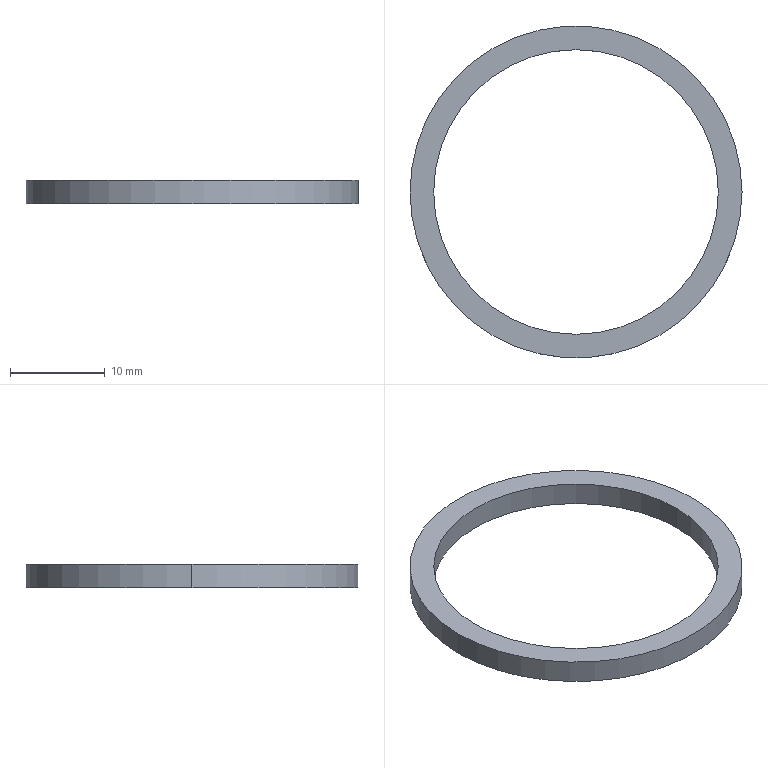Part | SolidWorks | features Extrusion 1 | 1 solid | 6 faces | box 35 x 35 x 2.5 mm | volume 638.136 mm3 | cylinder 4 | plane 2 | commonest cylinder face diameters 30 x2 35 x2
STEP:
#1=CARTESIAN_POINT('',(-15.,0.,2.5));
#2=VERTEX_POINT('',#1);
#3=CARTESIAN_POINT('',(15.,0.,2.5));
#4=VERTEX_POINT('',#3);
#5=CARTESIAN_POINT('',(0.,0.,2.5));
#6=DIRECTION('',(0.,0.,1.));
#7=DIRECTION('',(1.,0.,0.));
#8=AXIS2_PLACEMENT_3D('',#5,#6,#7);
#9=CIRCLE('',#8,15.);
#10=EDGE_CURVE('',#2,#4,#9,.T.);
#11=ORIENTED_EDGE('',*,*,#10,.T.);
#12=CARTESIAN_POINT('',(15.,0.,0.));
#13=VERTEX_POINT('',#12);
#14=CARTESIAN_POINT('',(15.,0.,2.5));
#15=DIRECTION('',(0.,0.,-1.));
#16=VECTOR('',#15,1000.);
#17=LINE('',#14,#16);
#18=EDGE_CURVE('',#4,#13,#17,.T.);
#19=ORIENTED_EDGE('',*,*,#18,.T.);
#20=CARTESIAN_POINT('',(-15.,0.,0.));
#21=VERTEX_POINT('',#20);
#22=CARTESIAN_POINT('',(0.,0.,0.));
#23=DIRECTION('',(0.,0.,1.));
#24=DIRECTION('',(1.,0.,0.));
#25=AXIS2_PLACEMENT_3D('',#22,#23,#24);
#26=CIRCLE('',#25,15.);
#27=EDGE_CURVE('',#21,#13,#26,.T.);
#28=ORIENTED_EDGE('',*,*,#27,.F.);
#29=CARTESIAN_POINT('',(-15.,0.,2.5));
#30=DIRECTION('',(0.,0.,-1.));
#31=VECTOR('',#30,1000.);
#32=LINE('',#29,#31);
#33=EDGE_CURVE('',#2,#21,#32,.T.);
#34=ORIENTED_EDGE('',*,*,#33,.F.);
#35=EDGE_LOOP('',(#11,#19,#28,#34));
#36=FACE_OUTER_BOUND('',#35,.T.);
#37=CARTESIAN_POINT('',(0.,0.,2.5));
#38=DIRECTION('',(0.,0.,-1.));
#39=DIRECTION('',(-1.,0.,0.));
#40=AXIS2_PLACEMENT_3D('',#37,#38,#39);
#41=CYLINDRICAL_SURFACE('',#40,15.);
#42=ADVANCED_FACE('',(#36),#41,.F.);
#43=CARTESIAN_POINT('',(17.5,0.,2.5));
#44=VERTEX_POINT('',#43);
#45=CARTESIAN_POINT('',(-17.5,0.,2.5));
#46=VERTEX_POINT('',#45);
#47=CARTESIAN_POINT('',(0.,0.,2.5));
#48=DIRECTION('',(0.,0.,1.));
#49=DIRECTION('',(1.,0.,0.));
#50=AXIS2_PLACEMENT_3D('',#47,#48,#49);
#51=CIRCLE('',#50,17.5);
#52=EDGE_CURVE('',#44,#46,#51,.T.);
#53=ORIENTED_EDGE('',*,*,#52,.F.);
#54=CARTESIAN_POINT('',(17.5,0.,0.));
#55=VERTEX_POINT('',#54);
#56=CARTESIAN_POINT('',(17.5,0.,2.5));
#57=DIRECTION('',(0.,0.,-1.));
#58=VECTOR('',#57,1000.);
#59=LINE('',#56,#58);
#60=EDGE_CURVE('',#44,#55,#59,.T.);
#61=ORIENTED_EDGE('',*,*,#60,.T.);
#62=CARTESIAN_POINT('',(-17.5,0.,0.));
#63=VERTEX_POINT('',#62);
#64=CARTESIAN_POINT('',(0.,0.,0.));
#65=DIRECTION('',(0.,0.,1.));
#66=DIRECTION('',(1.,0.,0.));
#67=AXIS2_PLACEMENT_3D('',#64,#65,#66);
#68=CIRCLE('',#67,17.5);
#69=EDGE_CURVE('',#55,#63,#68,.T.);
#70=ORIENTED_EDGE('',*,*,#69,.T.);
#71=CARTESIAN_POINT('',(-17.5,0.,2.5));
#72=DIRECTION('',(0.,0.,-1.));
#73=VECTOR('',#72,1000.);
#74=LINE('',#71,#73);
#75=EDGE_CURVE('',#46,#63,#74,.T.);
#76=ORIENTED_EDGE('',*,*,#75,.F.);
#77=EDGE_LOOP('',(#53,#61,#70,#76));
#78=FACE_OUTER_BOUND('',#77,.T.);
#79=CARTESIAN_POINT('',(0.,0.,2.5));
#80=DIRECTION('',(0.,0.,-1.));
#81=DIRECTION('',(-1.,0.,0.));
#82=AXIS2_PLACEMENT_3D('',#79,#80,#81);
#83=CYLINDRICAL_SURFACE('',#82,17.5);
#84=ADVANCED_FACE('',(#78),#83,.T.);
#85=CARTESIAN_POINT('',(0.,0.,2.5));
#86=DIRECTION('',(0.,0.,1.));
#87=DIRECTION('',(1.,0.,0.));
#88=AXIS2_PLACEMENT_3D('',#85,#86,#87);
#89=CIRCLE('',#88,17.5);
#90=EDGE_CURVE('',#46,#44,#89,.T.);
#91=ORIENTED_EDGE('',*,*,#90,.T.);
#92=ORIENTED_EDGE('',*,*,#52,.T.);
#93=EDGE_LOOP('',(#91,#92));
#94=FACE_OUTER_BOUND('',#93,.T.);
#95=ORIENTED_EDGE('',*,*,#10,.F.);
#96=CARTESIAN_POINT('',(0.,0.,2.5));
#97=DIRECTION('',(0.,0.,1.));
#98=DIRECTION('',(1.,0.,0.));
#99=AXIS2_PLACEMENT_3D('',#96,#97,#98);
#100=CIRCLE('',#99,15.);
#101=EDGE_CURVE('',#4,#2,#100,.T.);
#102=ORIENTED_EDGE('',*,*,#101,.F.);
#103=EDGE_LOOP('',(#95,#102));
#104=FACE_BOUND('',#103,.T.);
#105=CARTESIAN_POINT('',(0.,0.,2.5));
#106=DIRECTION('',(0.,0.,1.));
#107=DIRECTION('',(1.,0.,0.));
#108=AXIS2_PLACEMENT_3D('',#105,#106,#107);
#109=PLANE('',#108);
#110=ADVANCED_FACE('',(#94,#104),#109,.T.);
#111=CARTESIAN_POINT('',(0.,0.,0.));
#112=DIRECTION('',(0.,0.,1.));
#113=DIRECTION('',(1.,0.,0.));
#114=AXIS2_PLACEMENT_3D('',#111,#112,#113);
#115=CIRCLE('',#114,17.5);
#116=EDGE_CURVE('',#63,#55,#115,.T.);
#117=ORIENTED_EDGE('',*,*,#116,.F.);
#118=ORIENTED_EDGE('',*,*,#69,.F.);
#119=EDGE_LOOP('',(#117,#118));
#120=FACE_OUTER_BOUND('',#119,.T.);
#121=ORIENTED_EDGE('',*,*,#27,.T.);
#122=CARTESIAN_POINT('',(0.,0.,0.));
#123=DIRECTION('',(0.,0.,1.));
#124=DIRECTION('',(1.,0.,0.));
#125=AXIS2_PLACEMENT_3D('',#122,#123,#124);
#126=CIRCLE('',#125,15.);
#127=EDGE_CURVE('',#13,#21,#126,.T.);
#128=ORIENTED_EDGE('',*,*,#127,.T.);
#129=EDGE_LOOP('',(#121,#128));
#130=FACE_BOUND('',#129,.T.);
#131=CARTESIAN_POINT('',(0.,0.,0.));
#132=DIRECTION('',(0.,0.,1.));
#133=DIRECTION('',(1.,0.,0.));
#134=AXIS2_PLACEMENT_3D('',#131,#132,#133);
#135=PLANE('',#134);
#136=ADVANCED_FACE('',(#120,#130),#135,.F.);
#137=ORIENTED_EDGE('',*,*,#60,.F.);
#138=ORIENTED_EDGE('',*,*,#90,.F.);
#139=ORIENTED_EDGE('',*,*,#75,.T.);
#140=ORIENTED_EDGE('',*,*,#116,.T.);
#141=EDGE_LOOP('',(#137,#138,#139,#140));
#142=FACE_OUTER_BOUND('',#141,.T.);
#143=CARTESIAN_POINT('',(0.,0.,2.5));
#144=DIRECTION('',(0.,0.,-1.));
#145=DIRECTION('',(-1.,0.,0.));
#146=AXIS2_PLACEMENT_3D('',#143,#144,#145);
#147=CYLINDRICAL_SURFACE('',#146,17.5);
#148=ADVANCED_FACE('',(#142),#147,.T.);
#149=ORIENTED_EDGE('',*,*,#18,.F.);
#150=ORIENTED_EDGE('',*,*,#101,.T.);
#151=ORIENTED_EDGE('',*,*,#33,.T.);
#152=ORIENTED_EDGE('',*,*,#127,.F.);
#153=EDGE_LOOP('',(#149,#150,#151,#152));
#154=FACE_OUTER_BOUND('',#153,.T.);
#155=CARTESIAN_POINT('',(0.,0.,2.5));
#156=DIRECTION('',(0.,0.,-1.));
#157=DIRECTION('',(-1.,0.,0.));
#158=AXIS2_PLACEMENT_3D('',#155,#156,#157);
#159=CYLINDRICAL_SURFACE('',#158,15.);
#160=ADVANCED_FACE('',(#154),#159,.F.);
#161=CLOSED_SHELL('',(#42,#84,#110,#136,#148,#160));
#162=MANIFOLD_SOLID_BREP('',#161);
#163=CARTESIAN_POINT('',(0.,0.,0.));
#164=DIRECTION('',(0.,0.,1.));
#165=DIRECTION('',(1.,0.,0.));
#166=AXIS2_PLACEMENT_3D('',#163,#164,#165);
#167=(LENGTH_UNIT()NAMED_UNIT(*)SI_UNIT(.MILLI.,.METRE.));
#168=UNCERTAINTY_MEASURE_WITH_UNIT(LENGTH_MEASURE(0.00001),#167,'','');
#169=(NAMED_UNIT(*)PLANE_ANGLE_UNIT()SI_UNIT($,.RADIAN.));
#170=(NAMED_UNIT(*)SI_UNIT($,.STERADIAN.)SOLID_ANGLE_UNIT());
#171=(GEOMETRIC_REPRESENTATION_CONTEXT(3)GLOBAL_UNCERTAINTY_ASSIGNED_CONTEXT((#168))GLOBAL_UNIT_ASSIGNED_CONTEXT((#167,#169,#170))REPRESENTATION_CONTEXT('',''));
#172=ADVANCED_BREP_SHAPE_REPRESENTATION('',(#162,#166),#171);